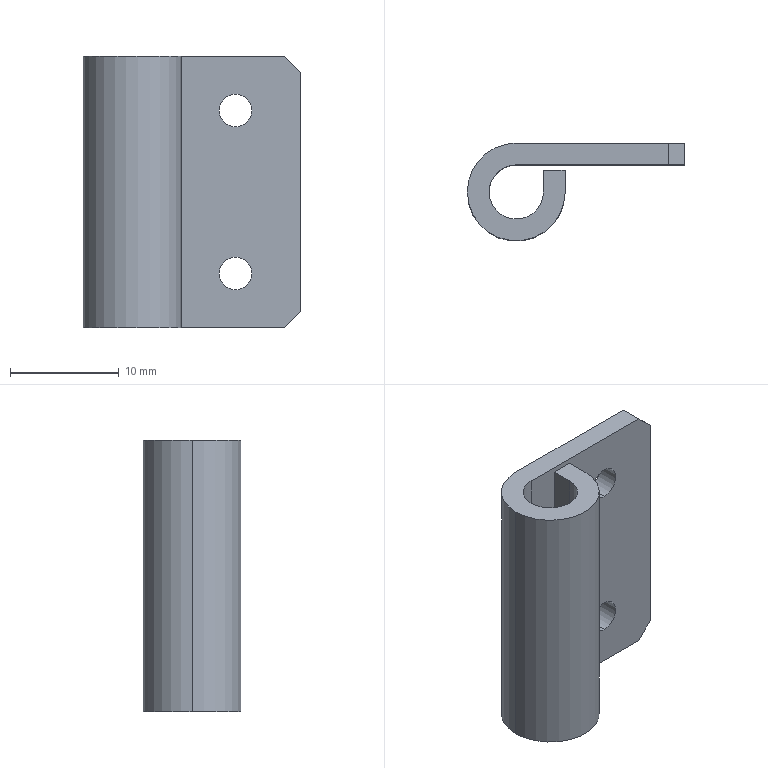Part | STEP file | 1 solid | 18 faces | box 20 x 9 x 25 mm | volume 1667 mm3 | plane 10 | cylinder 8 | commonest cylinder face diameters 3 x4 5 x2 9 x2
STEP:
#1=CARTESIAN_POINT('',(0.,0.,0.));
#2=DIRECTION('',(0.,0.,1.));
#3=DIRECTION('',(1.,0.,0.));
#4=AXIS2_PLACEMENT_3D('',#1,#2,#3);
#5=CARTESIAN_POINT('',(9.5,2.5,21.5));
#6=VERTEX_POINT('',#5);
#7=CARTESIAN_POINT('',(9.5,4.5,21.5));
#8=VERTEX_POINT('',#7);
#9=CARTESIAN_POINT('',(9.5,-4.5,21.5));
#10=DIRECTION('',(0.,1.,0.));
#11=VECTOR('',#10,1.);
#12=LINE('',#9,#11);
#13=CARTESIAN_POINT('',(9.5,-4.5,20.));
#14=DIRECTION('',(0.,1.,0.));
#15=DIRECTION('',(0.,0.,1.));
#16=AXIS2_PLACEMENT_3D('',#13,#14,#15);
#17=CYLINDRICAL_SURFACE('',#16,1.5);
#18=CARTESIAN_POINT('',(6.283,0.));
#19=DIRECTION('',(0.,1.));
#20=VECTOR('',#19,1.);
#21=LINE('',#18,#20);
#22=(GEOMETRIC_REPRESENTATION_CONTEXT(2)PARAMETRIC_REPRESENTATION_CONTEXT()REPRESENTATION_CONTEXT('',''));
#23=DEFINITIONAL_REPRESENTATION('',(#21),#22);
#24=PCURVE('',#17,#23);
#25=CARTESIAN_POINT('',(9.5,-4.5,20.));
#26=DIRECTION('',(0.,1.,0.));
#27=DIRECTION('',(0.,0.,1.));
#28=AXIS2_PLACEMENT_3D('',#25,#26,#27);
#29=CYLINDRICAL_SURFACE('',#28,1.5);
#30=CARTESIAN_POINT('',(0.,0.));
#31=DIRECTION('',(0.,1.));
#32=VECTOR('',#31,1.);
#33=LINE('',#30,#32);
#34=(GEOMETRIC_REPRESENTATION_CONTEXT(2)PARAMETRIC_REPRESENTATION_CONTEXT()REPRESENTATION_CONTEXT('',''));
#35=DEFINITIONAL_REPRESENTATION('',(#33),#34);
#36=PCURVE('',#29,#35);
#37=SURFACE_CURVE('',#12,(#24,#36),.PCURVE_S1.);
#38=EDGE_CURVE('',#6,#8,#37,.T.);
#39=ORIENTED_EDGE('',*,*,#38,.T.);
#40=CARTESIAN_POINT('',(9.5,4.5,18.5));
#41=VERTEX_POINT('',#40);
#42=CARTESIAN_POINT('',(9.5,4.5,20.));
#43=DIRECTION('',(0.,1.,0.));
#44=DIRECTION('',(0.,0.,-1.));
#45=AXIS2_PLACEMENT_3D('',#42,#43,#44);
#46=CIRCLE('',#45,1.5);
#47=CARTESIAN_POINT('',(3.142,9.));
#48=DIRECTION('',(1.,0.));
#49=VECTOR('',#48,1.);
#50=LINE('',#47,#49);
#51=(GEOMETRIC_REPRESENTATION_CONTEXT(2)PARAMETRIC_REPRESENTATION_CONTEXT()REPRESENTATION_CONTEXT('',''));
#52=DEFINITIONAL_REPRESENTATION('',(#50),#51);
#53=PCURVE('',#17,#52);
#54=CARTESIAN_POINT('',(0.,4.5,25.));
#55=DIRECTION('',(0.,-1.,0.));
#56=DIRECTION('',(0.,0.,-1.));
#57=AXIS2_PLACEMENT_3D('',#54,#55,#56);
#58=PLANE('',#57);
#59=CARTESIAN_POINT('',(6.5,9.5));
#60=CARTESIAN_POINT('',(6.5,6.902));
#61=CARTESIAN_POINT('',(4.25,8.201));
#62=CARTESIAN_POINT('',(2.,9.5));
#63=CARTESIAN_POINT('',(4.25,10.799));
#64=CARTESIAN_POINT('',(6.5,12.098));
#65=CARTESIAN_POINT('',(6.5,9.5));
#66=(BOUNDED_CURVE()B_SPLINE_CURVE(2,(#59,#60,#61,#62,#63,#64,#65),.UNSPECIFIED.,.T.,.F.)B_SPLINE_CURVE_WITH_KNOTS((1,2,2,2,2,1),(-2.094,0.,2.094,4.189,6.283,8.378),.UNSPECIFIED.)CURVE()GEOMETRIC_REPRESENTATION_ITEM()RATIONAL_B_SPLINE_CURVE((1.,0.5,1.,0.5,1.,0.5,1.))REPRESENTATION_ITEM(''));
#67=(GEOMETRIC_REPRESENTATION_CONTEXT(2)PARAMETRIC_REPRESENTATION_CONTEXT()REPRESENTATION_CONTEXT('',''));
#68=DEFINITIONAL_REPRESENTATION('',(#66),#67);
#69=PCURVE('',#58,#68);
#70=SURFACE_CURVE('',#46,(#53,#69),.PCURVE_S1.);
#71=EDGE_CURVE('',#41,#8,#70,.T.);
#72=ORIENTED_EDGE('',*,*,#71,.F.);
#73=CARTESIAN_POINT('',(9.5,2.5,18.5));
#74=VERTEX_POINT('',#73);
#75=CARTESIAN_POINT('',(9.5,-4.5,18.5));
#76=DIRECTION('',(0.,1.,0.));
#77=VECTOR('',#76,1.);
#78=LINE('',#75,#77);
#79=CARTESIAN_POINT('',(3.142,0.));
#80=DIRECTION('',(0.,1.));
#81=VECTOR('',#80,1.);
#82=LINE('',#79,#81);
#83=(GEOMETRIC_REPRESENTATION_CONTEXT(2)PARAMETRIC_REPRESENTATION_CONTEXT()REPRESENTATION_CONTEXT('',''));
#84=DEFINITIONAL_REPRESENTATION('',(#82),#83);
#85=PCURVE('',#17,#84);
#86=CARTESIAN_POINT('',(3.142,0.));
#87=DIRECTION('',(0.,1.));
#88=VECTOR('',#87,1.);
#89=LINE('',#86,#88);
#90=(GEOMETRIC_REPRESENTATION_CONTEXT(2)PARAMETRIC_REPRESENTATION_CONTEXT()REPRESENTATION_CONTEXT('',''));
#91=DEFINITIONAL_REPRESENTATION('',(#89),#90);
#92=PCURVE('',#29,#91);
#93=SURFACE_CURVE('',#78,(#85,#92),.PCURVE_S1.);
#94=EDGE_CURVE('',#74,#41,#93,.T.);
#95=ORIENTED_EDGE('',*,*,#94,.F.);
#96=CARTESIAN_POINT('',(9.5,2.5,20.));
#97=DIRECTION('',(0.,1.,0.));
#98=DIRECTION('',(-1.,0.,0.));
#99=AXIS2_PLACEMENT_3D('',#96,#97,#98);
#100=CIRCLE('',#99,1.5);
#101=CARTESIAN_POINT('',(-1.571,7.));
#102=DIRECTION('',(1.,0.));
#103=VECTOR('',#102,1.);
#104=LINE('',#101,#103);
#105=(GEOMETRIC_REPRESENTATION_CONTEXT(2)PARAMETRIC_REPRESENTATION_CONTEXT()REPRESENTATION_CONTEXT('',''));
#106=DEFINITIONAL_REPRESENTATION('',(#104),#105);
#107=PCURVE('',#17,#106);
#108=CARTESIAN_POINT('',(15.5,2.5,25.));
#109=DIRECTION('',(0.,1.,0.));
#110=DIRECTION('',(1.,0.,0.));
#111=AXIS2_PLACEMENT_3D('',#108,#109,#110);
#112=PLANE('',#111);
#113=CARTESIAN_POINT('',(-6.,5.));
#114=DIRECTION('',(-1.,0.));
#115=AXIS2_PLACEMENT_2D('',#113,#114);
#116=CIRCLE('',#115,1.5);
#117=(GEOMETRIC_REPRESENTATION_CONTEXT(2)PARAMETRIC_REPRESENTATION_CONTEXT()REPRESENTATION_CONTEXT('',''));
#118=DEFINITIONAL_REPRESENTATION('',(#116),#117);
#119=PCURVE('',#112,#118);
#120=SURFACE_CURVE('',#100,(#107,#119),.PCURVE_S1.);
#121=EDGE_CURVE('',#74,#6,#120,.T.);
#122=ORIENTED_EDGE('',*,*,#121,.T.);
#123=EDGE_LOOP('',(#39,#72,#95,#122));
#124=FACE_BOUND('',#123,.F.);
#125=ADVANCED_FACE('',(#124),#17,.F.);
#126=CARTESIAN_POINT('',(9.5,2.5,6.5));
#127=VERTEX_POINT('',#126);
#128=CARTESIAN_POINT('',(9.5,4.5,6.5));
#129=VERTEX_POINT('',#128);
#130=CARTESIAN_POINT('',(9.5,-4.5,6.5));
#131=DIRECTION('',(0.,1.,0.));
#132=VECTOR('',#131,1.);
#133=LINE('',#130,#132);
#134=CARTESIAN_POINT('',(9.5,-4.5,5.));
#135=DIRECTION('',(0.,1.,0.));
#136=DIRECTION('',(0.,0.,1.));
#137=AXIS2_PLACEMENT_3D('',#134,#135,#136);
#138=CYLINDRICAL_SURFACE('',#137,1.5);
#139=CARTESIAN_POINT('',(6.283,0.));
#140=DIRECTION('',(0.,1.));
#141=VECTOR('',#140,1.);
#142=LINE('',#139,#141);
#143=(GEOMETRIC_REPRESENTATION_CONTEXT(2)PARAMETRIC_REPRESENTATION_CONTEXT()REPRESENTATION_CONTEXT('',''));
#144=DEFINITIONAL_REPRESENTATION('',(#142),#143);
#145=PCURVE('',#138,#144);
#146=CARTESIAN_POINT('',(9.5,-4.5,5.));
#147=DIRECTION('',(0.,1.,0.));
#148=DIRECTION('',(0.,0.,1.));
#149=AXIS2_PLACEMENT_3D('',#146,#147,#148);
#150=CYLINDRICAL_SURFACE('',#149,1.5);
#151=CARTESIAN_POINT('',(0.,0.));
#152=DIRECTION('',(0.,1.));
#153=VECTOR('',#152,1.);
#154=LINE('',#151,#153);
#155=(GEOMETRIC_REPRESENTATION_CONTEXT(2)PARAMETRIC_REPRESENTATION_CONTEXT()REPRESENTATION_CONTEXT('',''));
#156=DEFINITIONAL_REPRESENTATION('',(#154),#155);
#157=PCURVE('',#150,#156);
#158=SURFACE_CURVE('',#133,(#145,#157),.PCURVE_S1.);
#159=EDGE_CURVE('',#127,#129,#158,.T.);
#160=ORIENTED_EDGE('',*,*,#159,.T.);
#161=CARTESIAN_POINT('',(9.5,4.5,3.5));
#162=VERTEX_POINT('',#161);
#163=CARTESIAN_POINT('',(9.5,4.5,5.));
#164=DIRECTION('',(0.,1.,0.));
#165=DIRECTION('',(0.,0.,1.));
#166=AXIS2_PLACEMENT_3D('',#163,#164,#165);
#167=CIRCLE('',#166,1.5);
#168=CARTESIAN_POINT('',(0.,9.));
#169=DIRECTION('',(1.,0.));
#170=VECTOR('',#169,1.);
#171=LINE('',#168,#170);
#172=(GEOMETRIC_REPRESENTATION_CONTEXT(2)PARAMETRIC_REPRESENTATION_CONTEXT()REPRESENTATION_CONTEXT('',''));
#173=DEFINITIONAL_REPRESENTATION('',(#171),#172);
#174=PCURVE('',#138,#173);
#175=CARTESIAN_POINT('',(18.5,9.5));
#176=CARTESIAN_POINT('',(18.5,12.098));
#177=CARTESIAN_POINT('',(20.75,10.799));
#178=CARTESIAN_POINT('',(23.,9.5));
#179=CARTESIAN_POINT('',(20.75,8.201));
#180=CARTESIAN_POINT('',(18.5,6.902));
#181=CARTESIAN_POINT('',(18.5,9.5));
#182=(BOUNDED_CURVE()B_SPLINE_CURVE(2,(#175,#176,#177,#178,#179,#180,#181),.UNSPECIFIED.,.T.,.F.)B_SPLINE_CURVE_WITH_KNOTS((1,2,2,2,2,1),(-2.094,0.,2.094,4.189,6.283,8.378),.UNSPECIFIED.)CURVE()GEOMETRIC_REPRESENTATION_ITEM()RATIONAL_B_SPLINE_CURVE((1.,0.5,1.,0.5,1.,0.5,1.))REPRESENTATION_ITEM(''));
#183=(GEOMETRIC_REPRESENTATION_CONTEXT(2)PARAMETRIC_REPRESENTATION_CONTEXT()REPRESENTATION_CONTEXT('',''));
#184=DEFINITIONAL_REPRESENTATION('',(#182),#183);
#185=PCURVE('',#58,#184);
#186=SURFACE_CURVE('',#167,(#174,#185),.PCURVE_S1.);
#187=EDGE_CURVE('',#162,#129,#186,.T.);
#188=ORIENTED_EDGE('',*,*,#187,.F.);
#189=CARTESIAN_POINT('',(9.5,2.5,3.5));
#190=VERTEX_POINT('',#189);
#191=CARTESIAN_POINT('',(9.5,-4.5,3.5));
#192=DIRECTION('',(0.,1.,0.));
#193=VECTOR('',#192,1.);
#194=LINE('',#191,#193);
#195=CARTESIAN_POINT('',(3.142,0.));
#196=DIRECTION('',(0.,1.));
#197=VECTOR('',#196,1.);
#198=LINE('',#195,#197);
#199=(GEOMETRIC_REPRESENTATION_CONTEXT(2)PARAMETRIC_REPRESENTATION_CONTEXT()REPRESENTATION_CONTEXT('',''));
#200=DEFINITIONAL_REPRESENTATION('',(#198),#199);
#201=PCURVE('',#138,#200);
#202=CARTESIAN_POINT('',(3.142,0.));
#203=DIRECTION('',(0.,1.));
#204=VECTOR('',#203,1.);
#205=LINE('',#202,#204);
#206=(GEOMETRIC_REPRESENTATION_CONTEXT(2)PARAMETRIC_REPRESENTATION_CONTEXT()REPRESENTATION_CONTEXT('',''));
#207=DEFINITIONAL_REPRESENTATION('',(#205),#206);
#208=PCURVE('',#150,#207);
#209=SURFACE_CURVE('',#194,(#201,#208),.PCURVE_S1.);
#210=EDGE_CURVE('',#190,#162,#209,.T.);
#211=ORIENTED_EDGE('',*,*,#210,.F.);
#212=CARTESIAN_POINT('',(9.5,2.5,5.));
#213=DIRECTION('',(0.,1.,0.));
#214=DIRECTION('',(-1.,0.,0.));
#215=AXIS2_PLACEMENT_3D('',#212,#213,#214);
#216=CIRCLE('',#215,1.5);
#217=CARTESIAN_POINT('',(-1.571,7.));
#218=DIRECTION('',(1.,0.));
#219=VECTOR('',#218,1.);
#220=LINE('',#217,#219);
#221=(GEOMETRIC_REPRESENTATION_CONTEXT(2)PARAMETRIC_REPRESENTATION_CONTEXT()REPRESENTATION_CONTEXT('',''));
#222=DEFINITIONAL_REPRESENTATION('',(#220),#221);
#223=PCURVE('',#138,#222);
#224=CARTESIAN_POINT('',(-6.,20.));
#225=DIRECTION('',(-1.,0.));
#226=AXIS2_PLACEMENT_2D('',#224,#225);
#227=CIRCLE('',#226,1.5);
#228=(GEOMETRIC_REPRESENTATION_CONTEXT(2)PARAMETRIC_REPRESENTATION_CONTEXT()REPRESENTATION_CONTEXT('',''));
#229=DEFINITIONAL_REPRESENTATION('',(#227),#228);
#230=PCURVE('',#112,#229);
#231=SURFACE_CURVE('',#216,(#223,#230),.PCURVE_S1.);
#232=EDGE_CURVE('',#190,#127,#231,.T.);
#233=ORIENTED_EDGE('',*,*,#232,.T.);
#234=EDGE_LOOP('',(#160,#188,#211,#233));
#235=FACE_BOUND('',#234,.F.);
#236=ADVANCED_FACE('',(#235),#138,.F.);
#237=CARTESIAN_POINT('',(0.,2.5,25.));
#238=VERTEX_POINT('',#237);
#239=CARTESIAN_POINT('',(0.,2.5,0.));
#240=VERTEX_POINT('',#239);
#241=CARTESIAN_POINT('',(0.,2.5,25.));
#242=DIRECTION('',(0.,0.,-1.));
#243=VECTOR('',#242,1.);
#244=LINE('',#241,#243);
#245=CARTESIAN_POINT('',(0.,0.,25.));
#246=DIRECTION('',(0.,0.,-1.));
#247=DIRECTION('',(-1.,0.,0.));
#248=AXIS2_PLACEMENT_3D('',#245,#246,#247);
#249=CYLINDRICAL_SURFACE('',#248,2.5);
#250=CARTESIAN_POINT('',(1.571,0.));
#251=DIRECTION('',(0.,1.));
#252=VECTOR('',#251,1.);
#253=LINE('',#250,#252);
#254=(GEOMETRIC_REPRESENTATION_CONTEXT(2)PARAMETRIC_REPRESENTATION_CONTEXT()REPRESENTATION_CONTEXT('',''));
#255=DEFINITIONAL_REPRESENTATION('',(#253),#254);
#256=PCURVE('',#249,#255);
#257=CARTESIAN_POINT('',(-15.5,0.));
#258=DIRECTION('',(0.,1.));
#259=VECTOR('',#258,1.);
#260=LINE('',#257,#259);
#261=(GEOMETRIC_REPRESENTATION_CONTEXT(2)PARAMETRIC_REPRESENTATION_CONTEXT()REPRESENTATION_CONTEXT('',''));
#262=DEFINITIONAL_REPRESENTATION('',(#260),#261);
#263=PCURVE('',#112,#262);
#264=SURFACE_CURVE('',#244,(#256,#263),.PCURVE_S1.);
#265=EDGE_CURVE('',#238,#240,#264,.T.);
#266=ORIENTED_EDGE('',*,*,#265,.T.);
#267=CARTESIAN_POINT('',(-2.5,0.,0.));
#268=VERTEX_POINT('',#267);
#269=CARTESIAN_POINT('',(0.,0.,0.));
#270=DIRECTION('',(0.,0.,-1.));
#271=DIRECTION('',(1.,0.,0.));
#272=AXIS2_PLACEMENT_3D('',#269,#270,#271);
#273=CIRCLE('',#272,2.5);
#274=CARTESIAN_POINT('',(-3.142,25.));
#275=DIRECTION('',(1.,0.));
#276=VECTOR('',#275,1.);
#277=LINE('',#274,#276);
#278=(GEOMETRIC_REPRESENTATION_CONTEXT(2)PARAMETRIC_REPRESENTATION_CONTEXT()REPRESENTATION_CONTEXT('',''));
#279=DEFINITIONAL_REPRESENTATION('',(#277),#278);
#280=PCURVE('',#249,#279);
#281=CARTESIAN_POINT('',(0.,0.,0.));
#282=DIRECTION('',(0.,0.,1.));
#283=DIRECTION('',(1.,0.,0.));
#284=AXIS2_PLACEMENT_3D('',#281,#282,#283);
#285=PLANE('',#284);
#286=CARTESIAN_POINT('',(2.5,0.));
#287=CARTESIAN_POINT('',(2.5,-4.33));
#288=CARTESIAN_POINT('',(-1.25,-2.165));
#289=CARTESIAN_POINT('',(-5.,0.));
#290=CARTESIAN_POINT('',(-1.25,2.165));
#291=CARTESIAN_POINT('',(2.5,4.33));
#292=CARTESIAN_POINT('',(2.5,0.));
#293=(BOUNDED_CURVE()B_SPLINE_CURVE(2,(#286,#287,#288,#289,#290,#291,#292),.UNSPECIFIED.,.T.,.F.)B_SPLINE_CURVE_WITH_KNOTS((1,2,2,2,2,1),(-2.094,0.,2.094,4.189,6.283,8.378),.UNSPECIFIED.)CURVE()GEOMETRIC_REPRESENTATION_ITEM()RATIONAL_B_SPLINE_CURVE((1.,0.5,1.,0.5,1.,0.5,1.))REPRESENTATION_ITEM(''));
#294=(GEOMETRIC_REPRESENTATION_CONTEXT(2)PARAMETRIC_REPRESENTATION_CONTEXT()REPRESENTATION_CONTEXT('',''));
#295=DEFINITIONAL_REPRESENTATION('',(#293),#294);
#296=PCURVE('',#285,#295);
#297=SURFACE_CURVE('',#273,(#280,#296),.PCURVE_S1.);
#298=EDGE_CURVE('',#268,#240,#297,.T.);
#299=ORIENTED_EDGE('',*,*,#298,.F.);
#300=CARTESIAN_POINT('',(-2.5,0.,25.));
#301=VERTEX_POINT('',#300);
#302=CARTESIAN_POINT('',(-2.5,0.,25.));
#303=DIRECTION('',(0.,0.,-1.));
#304=VECTOR('',#303,1.);
#305=LINE('',#302,#304);
#306=CARTESIAN_POINT('',(0.,0.));
#307=DIRECTION('',(0.,1.));
#308=VECTOR('',#307,1.);
#309=LINE('',#306,#308);
#310=(GEOMETRIC_REPRESENTATION_CONTEXT(2)PARAMETRIC_REPRESENTATION_CONTEXT()REPRESENTATION_CONTEXT('',''));
#311=DEFINITIONAL_REPRESENTATION('',(#309),#310);
#312=PCURVE('',#249,#311);
#313=CARTESIAN_POINT('',(0.,0.,25.));
#314=DIRECTION('',(0.,0.,-1.));
#315=DIRECTION('',(-1.,0.,0.));
#316=AXIS2_PLACEMENT_3D('',#313,#314,#315);
#317=CYLINDRICAL_SURFACE('',#316,2.5);
#318=CARTESIAN_POINT('',(6.283,0.));
#319=DIRECTION('',(0.,1.));
#320=VECTOR('',#319,1.);
#321=LINE('',#318,#320);
#322=(GEOMETRIC_REPRESENTATION_CONTEXT(2)PARAMETRIC_REPRESENTATION_CONTEXT()REPRESENTATION_CONTEXT('',''));
#323=DEFINITIONAL_REPRESENTATION('',(#321),#322);
#324=PCURVE('',#317,#323);
#325=SURFACE_CURVE('',#305,(#312,#324),.PCURVE_S1.);
#326=EDGE_CURVE('',#301,#268,#325,.T.);
#327=ORIENTED_EDGE('',*,*,#326,.F.);
#328=CARTESIAN_POINT('',(0.,0.,25.));
#329=DIRECTION('',(0.,0.,-1.));
#330=DIRECTION('',(1.,0.,0.));
#331=AXIS2_PLACEMENT_3D('',#328,#329,#330);
#332=CIRCLE('',#331,2.5);
#333=CARTESIAN_POINT('',(-3.142,0.));
#334=DIRECTION('',(1.,0.));
#335=VECTOR('',#334,1.);
#336=LINE('',#333,#335);
#337=(GEOMETRIC_REPRESENTATION_CONTEXT(2)PARAMETRIC_REPRESENTATION_CONTEXT()REPRESENTATION_CONTEXT('',''));
#338=DEFINITIONAL_REPRESENTATION('',(#336),#337);
#339=PCURVE('',#249,#338);
#340=CARTESIAN_POINT('',(0.,0.,25.));
#341=DIRECTION('',(0.,0.,1.));
#342=DIRECTION('',(1.,0.,0.));
#343=AXIS2_PLACEMENT_3D('',#340,#341,#342);
#344=PLANE('',#343);
#345=CARTESIAN_POINT('',(2.5,0.));
#346=CARTESIAN_POINT('',(2.5,-4.33));
#347=CARTESIAN_POINT('',(-1.25,-2.165));
#348=CARTESIAN_POINT('',(-5.,0.));
#349=CARTESIAN_POINT('',(-1.25,2.165));
#350=CARTESIAN_POINT('',(2.5,4.33));
#351=CARTESIAN_POINT('',(2.5,0.));
#352=(BOUNDED_CURVE()B_SPLINE_CURVE(2,(#345,#346,#347,#348,#349,#350,#351),.UNSPECIFIED.,.T.,.F.)B_SPLINE_CURVE_WITH_KNOTS((1,2,2,2,2,1),(-2.094,0.,2.094,4.189,6.283,8.378),.UNSPECIFIED.)CURVE()GEOMETRIC_REPRESENTATION_ITEM()RATIONAL_B_SPLINE_CURVE((1.,0.5,1.,0.5,1.,0.5,1.))REPRESENTATION_ITEM(''));
#353=(GEOMETRIC_REPRESENTATION_CONTEXT(2)PARAMETRIC_REPRESENTATION_CONTEXT()REPRESENTATION_CONTEXT('',''));
#354=DEFINITIONAL_REPRESENTATION('',(#352),#353);
#355=PCURVE('',#344,#354);
#356=SURFACE_CURVE('',#332,(#339,#355),.PCURVE_S1.);
#357=EDGE_CURVE('',#301,#238,#356,.T.);
#358=ORIENTED_EDGE('',*,*,#357,.T.);
#359=EDGE_LOOP('',(#266,#299,#327,#358));
#360=FACE_BOUND('',#359,.F.);
#361=ADVANCED_FACE('',(#360),#249,.F.);
#362=CARTESIAN_POINT('',(-4.5,0.,25.));
#363=VERTEX_POINT('',#362);
#364=CARTESIAN_POINT('',(4.5,0.,25.));
#365=VERTEX_POINT('',#364);
#366=CARTESIAN_POINT('',(0.,0.,25.));
#367=DIRECTION('',(0.,0.,1.));
#368=DIRECTION('',(1.,0.,0.));
#369=AXIS2_PLACEMENT_3D('',#366,#367,#368);
#370=CIRCLE('',#369,4.5);
#371=CARTESIAN_POINT('',(0.,0.,25.));
#372=DIRECTION('',(0.,0.,-1.));
#373=DIRECTION('',(-1.,0.,0.));
#374=AXIS2_PLACEMENT_3D('',#371,#372,#373);
#375=CYLINDRICAL_SURFACE('',#374,4.5);
#376=CARTESIAN_POINT('',(9.425,0.));
#377=DIRECTION('',(-1.,0.));
#378=VECTOR('',#377,1.);
#379=LINE('',#376,#378);
#380=(GEOMETRIC_REPRESENTATION_CONTEXT(2)PARAMETRIC_REPRESENTATION_CONTEXT()REPRESENTATION_CONTEXT('',''));
#381=DEFINITIONAL_REPRESENTATION('',(#379),#380);
#382=PCURVE('',#375,#381);
#383=CARTESIAN_POINT('',(0.,0.));
#384=DIRECTION('',(1.,0.));
#385=AXIS2_PLACEMENT_2D('',#383,#384);
#386=CIRCLE('',#385,4.5);
#387=(GEOMETRIC_REPRESENTATION_CONTEXT(2)PARAMETRIC_REPRESENTATION_CONTEXT()REPRESENTATION_CONTEXT('',''));
#388=DEFINITIONAL_REPRESENTATION('',(#386),#387);
#389=PCURVE('',#344,#388);
#390=SURFACE_CURVE('',#370,(#382,#389),.PCURVE_S1.);
#391=EDGE_CURVE('',#363,#365,#390,.T.);
#392=ORIENTED_EDGE('',*,*,#391,.F.);
#393=CARTESIAN_POINT('',(-4.5,0.,0.));
#394=VERTEX_POINT('',#393);
#395=CARTESIAN_POINT('',(-4.5,0.,25.));
#396=DIRECTION('',(0.,0.,-1.));
#397=VECTOR('',#396,1.);
#398=LINE('',#395,#397);
#399=CARTESIAN_POINT('',(6.283,0.));
#400=DIRECTION('',(0.,1.));
#401=VECTOR('',#400,1.);
#402=LINE('',#399,#401);
#403=(GEOMETRIC_REPRESENTATION_CONTEXT(2)PARAMETRIC_REPRESENTATION_CONTEXT()REPRESENTATION_CONTEXT('',''));
#404=DEFINITIONAL_REPRESENTATION('',(#402),#403);
#405=PCURVE('',#375,#404);
#406=CARTESIAN_POINT('',(0.,0.,25.));
#407=DIRECTION('',(0.,0.,-1.));
#408=DIRECTION('',(-1.,0.,0.));
#409=AXIS2_PLACEMENT_3D('',#406,#407,#408);
#410=CYLINDRICAL_SURFACE('',#409,4.5);
#411=CARTESIAN_POINT('',(0.,0.));
#412=DIRECTION('',(0.,1.));
#413=VECTOR('',#412,1.);
#414=LINE('',#411,#413);
#415=(GEOMETRIC_REPRESENTATION_CONTEXT(2)PARAMETRIC_REPRESENTATION_CONTEXT()REPRESENTATION_CONTEXT('',''));
#416=DEFINITIONAL_REPRESENTATION('',(#414),#415);
#417=PCURVE('',#410,#416);
#418=SURFACE_CURVE('',#398,(#405,#417),.PCURVE_S1.);
#419=EDGE_CURVE('',#363,#394,#418,.T.);
#420=ORIENTED_EDGE('',*,*,#419,.T.);
#421=CARTESIAN_POINT('',(4.5,0.,0.));
#422=VERTEX_POINT('',#421);
#423=CARTESIAN_POINT('',(0.,0.,0.));
#424=DIRECTION('',(0.,0.,1.));
#425=DIRECTION('',(1.,0.,0.));
#426=AXIS2_PLACEMENT_3D('',#423,#424,#425);
#427=CIRCLE('',#426,4.5);
#428=CARTESIAN_POINT('',(9.425,25.));
#429=DIRECTION('',(-1.,0.));
#430=VECTOR('',#429,1.);
#431=LINE('',#428,#430);
#432=(GEOMETRIC_REPRESENTATION_CONTEXT(2)PARAMETRIC_REPRESENTATION_CONTEXT()REPRESENTATION_CONTEXT('',''));
#433=DEFINITIONAL_REPRESENTATION('',(#431),#432);
#434=PCURVE('',#375,#433);
#435=CARTESIAN_POINT('',(0.,0.));
#436=DIRECTION('',(1.,0.));
#437=AXIS2_PLACEMENT_2D('',#435,#436);
#438=CIRCLE('',#437,4.5);
#439=(GEOMETRIC_REPRESENTATION_CONTEXT(2)PARAMETRIC_REPRESENTATION_CONTEXT()REPRESENTATION_CONTEXT('',''));
#440=DEFINITIONAL_REPRESENTATION('',(#438),#439);
#441=PCURVE('',#285,#440);
#442=SURFACE_CURVE('',#427,(#434,#441),.PCURVE_S1.);
#443=EDGE_CURVE('',#394,#422,#442,.T.);
#444=ORIENTED_EDGE('',*,*,#443,.T.);
#445=CARTESIAN_POINT('',(4.5,0.,25.));
#446=DIRECTION('',(0.,0.,-1.));
#447=VECTOR('',#446,1.);
#448=LINE('',#445,#447);
#449=CARTESIAN_POINT('',(3.142,0.));
#450=DIRECTION('',(0.,1.));
#451=VECTOR('',#450,1.);
#452=LINE('',#449,#451);
#453=(GEOMETRIC_REPRESENTATION_CONTEXT(2)PARAMETRIC_REPRESENTATION_CONTEXT()REPRESENTATION_CONTEXT('',''));
#454=DEFINITIONAL_REPRESENTATION('',(#452),#453);
#455=PCURVE('',#375,#454);
#456=CARTESIAN_POINT('',(4.5,0.,25.));
#457=DIRECTION('',(-1.,0.,0.));
#458=DIRECTION('',(0.,0.,1.));
#459=AXIS2_PLACEMENT_3D('',#456,#457,#458);
#460=PLANE('',#459);
#461=CARTESIAN_POINT('',(0.,0.));
#462=DIRECTION('',(-1.,0.));
#463=VECTOR('',#462,1.);
#464=LINE('',#461,#463);
#465=(GEOMETRIC_REPRESENTATION_CONTEXT(2)PARAMETRIC_REPRESENTATION_CONTEXT()REPRESENTATION_CONTEXT('',''));
#466=DEFINITIONAL_REPRESENTATION('',(#464),#465);
#467=PCURVE('',#460,#466);
#468=SURFACE_CURVE('',#448,(#455,#467),.PCURVE_S1.);
#469=EDGE_CURVE('',#365,#422,#468,.T.);
#470=ORIENTED_EDGE('',*,*,#469,.F.);
#471=EDGE_LOOP('',(#392,#420,#444,#470));
#472=FACE_BOUND('',#471,.T.);
#473=ADVANCED_FACE('',(#472),#375,.T.);
#474=CARTESIAN_POINT('',(15.5,2.5,23.5));
#475=VERTEX_POINT('',#474);
#476=CARTESIAN_POINT('',(15.5,4.5,23.5));
#477=VERTEX_POINT('',#476);
#478=CARTESIAN_POINT('',(15.5,-4.5,23.5));
#479=DIRECTION('',(0.,1.,0.));
#480=VECTOR('',#479,1.);
#481=LINE('',#478,#480);
#482=CARTESIAN_POINT('',(14.,-4.5,25.));
#483=DIRECTION('',(-0.7071,0.,-0.7071));
#484=DIRECTION('',(-0.7071,0.,0.7071));
#485=AXIS2_PLACEMENT_3D('',#482,#483,#484);
#486=PLANE('',#485);
#487=CARTESIAN_POINT('',(-2.121,0.));
#488=DIRECTION('',(0.,1.));
#489=VECTOR('',#488,1.);
#490=LINE('',#487,#489);
#491=(GEOMETRIC_REPRESENTATION_CONTEXT(2)PARAMETRIC_REPRESENTATION_CONTEXT()REPRESENTATION_CONTEXT('',''));
#492=DEFINITIONAL_REPRESENTATION('',(#490),#491);
#493=PCURVE('',#486,#492);
#494=CARTESIAN_POINT('',(15.5,4.5,25.));
#495=DIRECTION('',(-1.,0.,0.));
#496=DIRECTION('',(0.,1.,0.));
#497=AXIS2_PLACEMENT_3D('',#494,#495,#496);
#498=PLANE('',#497);
#499=CARTESIAN_POINT('',(-9.,1.5));
#500=DIRECTION('',(1.,0.));
#501=VECTOR('',#500,1.);
#502=LINE('',#499,#501);
#503=(GEOMETRIC_REPRESENTATION_CONTEXT(2)PARAMETRIC_REPRESENTATION_CONTEXT()REPRESENTATION_CONTEXT('',''));
#504=DEFINITIONAL_REPRESENTATION('',(#502),#503);
#505=PCURVE('',#498,#504);
#506=SURFACE_CURVE('',#481,(#493,#505),.PCURVE_S1.);
#507=EDGE_CURVE('',#475,#477,#506,.T.);
#508=ORIENTED_EDGE('',*,*,#507,.T.);
#509=CARTESIAN_POINT('',(14.,4.5,25.));
#510=VERTEX_POINT('',#509);
#511=CARTESIAN_POINT('',(14.,4.5,25.));
#512=DIRECTION('',(-0.7071,0.,0.7071));
#513=VECTOR('',#512,1.);
#514=LINE('',#511,#513);
#515=CARTESIAN_POINT('',(0.,9.));
#516=DIRECTION('',(1.,0.));
#517=VECTOR('',#516,1.);
#518=LINE('',#515,#517);
#519=(GEOMETRIC_REPRESENTATION_CONTEXT(2)PARAMETRIC_REPRESENTATION_CONTEXT()REPRESENTATION_CONTEXT('',''));
#520=DEFINITIONAL_REPRESENTATION('',(#518),#519);
#521=PCURVE('',#486,#520);
#522=CARTESIAN_POINT('',(0.,14.));
#523=DIRECTION('',(-0.7071,-0.7071));
#524=VECTOR('',#523,1.);
#525=LINE('',#522,#524);
#526=(GEOMETRIC_REPRESENTATION_CONTEXT(2)PARAMETRIC_REPRESENTATION_CONTEXT()REPRESENTATION_CONTEXT('',''));
#527=DEFINITIONAL_REPRESENTATION('',(#525),#526);
#528=PCURVE('',#58,#527);
#529=SURFACE_CURVE('',#514,(#521,#528),.PCURVE_S1.);
#530=EDGE_CURVE('',#477,#510,#529,.T.);
#531=ORIENTED_EDGE('',*,*,#530,.T.);
#532=CARTESIAN_POINT('',(14.,2.5,25.));
#533=VERTEX_POINT('',#532);
#534=CARTESIAN_POINT('',(14.,0.,25.));
#535=DIRECTION('',(0.,-1.,0.));
#536=VECTOR('',#535,1.);
#537=LINE('',#534,#536);
#538=CARTESIAN_POINT('',(0.,4.5));
#539=DIRECTION('',(0.,-1.));
#540=VECTOR('',#539,1.);
#541=LINE('',#538,#540);
#542=(GEOMETRIC_REPRESENTATION_CONTEXT(2)PARAMETRIC_REPRESENTATION_CONTEXT()REPRESENTATION_CONTEXT('',''));
#543=DEFINITIONAL_REPRESENTATION('',(#541),#542);
#544=PCURVE('',#486,#543);
#545=CARTESIAN_POINT('',(14.,0.));
#546=DIRECTION('',(0.,-1.));
#547=VECTOR('',#546,1.);
#548=LINE('',#545,#547);
#549=(GEOMETRIC_REPRESENTATION_CONTEXT(2)PARAMETRIC_REPRESENTATION_CONTEXT()REPRESENTATION_CONTEXT('',''));
#550=DEFINITIONAL_REPRESENTATION('',(#548),#549);
#551=PCURVE('',#344,#550);
#552=SURFACE_CURVE('',#537,(#544,#551),.PCURVE_S1.);
#553=EDGE_CURVE('',#510,#533,#552,.T.);
#554=ORIENTED_EDGE('',*,*,#553,.T.);
#555=CARTESIAN_POINT('',(14.75,2.5,24.25));
#556=DIRECTION('',(-0.7071,0.,0.7071));
#557=VECTOR('',#556,1.);
#558=LINE('',#555,#557);
#559=CARTESIAN_POINT('',(-1.061,7.));
#560=DIRECTION('',(1.,0.));
#561=VECTOR('',#560,1.);
#562=LINE('',#559,#561);
#563=(GEOMETRIC_REPRESENTATION_CONTEXT(2)PARAMETRIC_REPRESENTATION_CONTEXT()REPRESENTATION_CONTEXT('',''));
#564=DEFINITIONAL_REPRESENTATION('',(#562),#563);
#565=PCURVE('',#486,#564);
#566=CARTESIAN_POINT('',(-0.75,0.75));
#567=DIRECTION('',(-0.7071,-0.7071));
#568=VECTOR('',#567,1.);
#569=LINE('',#566,#568);
#570=(GEOMETRIC_REPRESENTATION_CONTEXT(2)PARAMETRIC_REPRESENTATION_CONTEXT()REPRESENTATION_CONTEXT('',''));
#571=DEFINITIONAL_REPRESENTATION('',(#569),#570);
#572=PCURVE('',#112,#571);
#573=SURFACE_CURVE('',#558,(#565,#572),.PCURVE_S1.);
#574=EDGE_CURVE('',#475,#533,#573,.T.);
#575=ORIENTED_EDGE('',*,*,#574,.F.);
#576=EDGE_LOOP('',(#508,#531,#554,#575));
#577=FACE_BOUND('',#576,.T.);
#578=ADVANCED_FACE('',(#577),#486,.F.);
#579=CARTESIAN_POINT('',(14.,4.5,0.));
#580=VERTEX_POINT('',#579);
#581=CARTESIAN_POINT('',(14.,2.5,0.));
#582=VERTEX_POINT('',#581);
#583=CARTESIAN_POINT('',(14.,0.,0.));
#584=DIRECTION('',(0.,-1.,0.));
#585=VECTOR('',#584,1.);
#586=LINE('',#583,#585);
#587=CARTESIAN_POINT('',(14.,-4.5,0.));
#588=DIRECTION('',(-0.7071,0.,0.7071));
#589=DIRECTION('',(0.,1.,0.));
#590=AXIS2_PLACEMENT_3D('',#587,#588,#589);
#591=PLANE('',#590);
#592=CARTESIAN_POINT('',(4.5,0.));
#593=DIRECTION('',(-1.,0.));
#594=VECTOR('',#593,1.);
#595=LINE('',#592,#594);
#596=(GEOMETRIC_REPRESENTATION_CONTEXT(2)PARAMETRIC_REPRESENTATION_CONTEXT()REPRESENTATION_CONTEXT('',''));
#597=DEFINITIONAL_REPRESENTATION('',(#595),#596);
#598=PCURVE('',#591,#597);
#599=CARTESIAN_POINT('',(14.,0.));
#600=DIRECTION('',(0.,-1.));
#601=VECTOR('',#600,1.);
#602=LINE('',#599,#601);
#603=(GEOMETRIC_REPRESENTATION_CONTEXT(2)PARAMETRIC_REPRESENTATION_CONTEXT()REPRESENTATION_CONTEXT('',''));
#604=DEFINITIONAL_REPRESENTATION('',(#602),#603);
#605=PCURVE('',#285,#604);
#606=SURFACE_CURVE('',#586,(#598,#605),.PCURVE_S1.);
#607=EDGE_CURVE('',#580,#582,#606,.T.);
#608=ORIENTED_EDGE('',*,*,#607,.F.);
#609=CARTESIAN_POINT('',(15.5,4.5,1.5));
#610=VERTEX_POINT('',#609);
#611=CARTESIAN_POINT('',(14.,4.5,0.));
#612=DIRECTION('',(0.7071,0.,0.7071));
#613=VECTOR('',#612,1.);
#614=LINE('',#611,#613);
#615=CARTESIAN_POINT('',(9.,0.));
#616=DIRECTION('',(0.,-1.));
#617=VECTOR('',#616,1.);
#618=LINE('',#615,#617);
#619=(GEOMETRIC_REPRESENTATION_CONTEXT(2)PARAMETRIC_REPRESENTATION_CONTEXT()REPRESENTATION_CONTEXT('',''));
#620=DEFINITIONAL_REPRESENTATION('',(#618),#619);
#621=PCURVE('',#591,#620);
#622=CARTESIAN_POINT('',(25.,14.));
#623=DIRECTION('',(-0.7071,0.7071));
#624=VECTOR('',#623,1.);
#625=LINE('',#622,#624);
#626=(GEOMETRIC_REPRESENTATION_CONTEXT(2)PARAMETRIC_REPRESENTATION_CONTEXT()REPRESENTATION_CONTEXT('',''));
#627=DEFINITIONAL_REPRESENTATION('',(#625),#626);
#628=PCURVE('',#58,#627);
#629=SURFACE_CURVE('',#614,(#621,#628),.PCURVE_S1.);
#630=EDGE_CURVE('',#580,#610,#629,.T.);
#631=ORIENTED_EDGE('',*,*,#630,.T.);
#632=CARTESIAN_POINT('',(15.5,2.5,1.5));
#633=VERTEX_POINT('',#632);
#634=CARTESIAN_POINT('',(15.5,-4.5,1.5));
#635=DIRECTION('',(0.,1.,0.));
#636=VECTOR('',#635,1.);
#637=LINE('',#634,#636);
#638=CARTESIAN_POINT('',(0.,-2.121));
#639=DIRECTION('',(1.,0.));
#640=VECTOR('',#639,1.);
#641=LINE('',#638,#640);
#642=(GEOMETRIC_REPRESENTATION_CONTEXT(2)PARAMETRIC_REPRESENTATION_CONTEXT()REPRESENTATION_CONTEXT('',''));
#643=DEFINITIONAL_REPRESENTATION('',(#641),#642);
#644=PCURVE('',#591,#643);
#645=CARTESIAN_POINT('',(-9.,23.5));
#646=DIRECTION('',(1.,0.));
#647=VECTOR('',#646,1.);
#648=LINE('',#645,#647);
#649=(GEOMETRIC_REPRESENTATION_CONTEXT(2)PARAMETRIC_REPRESENTATION_CONTEXT()REPRESENTATION_CONTEXT('',''));
#650=DEFINITIONAL_REPRESENTATION('',(#648),#649);
#651=PCURVE('',#498,#650);
#652=SURFACE_CURVE('',#637,(#644,#651),.PCURVE_S1.);
#653=EDGE_CURVE('',#633,#610,#652,.T.);
#654=ORIENTED_EDGE('',*,*,#653,.F.);
#655=CARTESIAN_POINT('',(27.25,2.5,13.25));
#656=DIRECTION('',(0.7071,0.,0.7071));
#657=VECTOR('',#656,1.);
#658=LINE('',#655,#657);
#659=CARTESIAN_POINT('',(7.,-18.738));
#660=DIRECTION('',(0.,-1.));
#661=VECTOR('',#660,1.);
#662=LINE('',#659,#661);
#663=(GEOMETRIC_REPRESENTATION_CONTEXT(2)PARAMETRIC_REPRESENTATION_CONTEXT()REPRESENTATION_CONTEXT('',''));
#664=DEFINITIONAL_REPRESENTATION('',(#662),#663);
#665=PCURVE('',#591,#664);
#666=CARTESIAN_POINT('',(11.75,11.75));
#667=DIRECTION('',(0.7071,-0.7071));
#668=VECTOR('',#667,1.);
#669=LINE('',#666,#668);
#670=(GEOMETRIC_REPRESENTATION_CONTEXT(2)PARAMETRIC_REPRESENTATION_CONTEXT()REPRESENTATION_CONTEXT('',''));
#671=DEFINITIONAL_REPRESENTATION('',(#669),#670);
#672=PCURVE('',#112,#671);
#673=SURFACE_CURVE('',#658,(#665,#672),.PCURVE_S1.);
#674=EDGE_CURVE('',#582,#633,#673,.T.);
#675=ORIENTED_EDGE('',*,*,#674,.F.);
#676=EDGE_LOOP('',(#608,#631,#654,#675));
#677=FACE_BOUND('',#676,.T.);
#678=ADVANCED_FACE('',(#677),#591,.F.);
#679=CARTESIAN_POINT('',(0.,4.5,0.));
#680=VERTEX_POINT('',#679);
#681=CARTESIAN_POINT('',(0.,4.5,0.));
#682=DIRECTION('',(-1.,0.,0.));
#683=VECTOR('',#682,1.);
#684=LINE('',#681,#683);
#685=CARTESIAN_POINT('',(0.,4.5));
#686=DIRECTION('',(-1.,0.));
#687=VECTOR('',#686,1.);
#688=LINE('',#685,#687);
#689=(GEOMETRIC_REPRESENTATION_CONTEXT(2)PARAMETRIC_REPRESENTATION_CONTEXT()REPRESENTATION_CONTEXT('',''));
#690=DEFINITIONAL_REPRESENTATION('',(#688),#689);
#691=PCURVE('',#285,#690);
#692=CARTESIAN_POINT('',(25.,0.));
#693=DIRECTION('',(0.,-1.));
#694=VECTOR('',#693,1.);
#695=LINE('',#692,#694);
#696=(GEOMETRIC_REPRESENTATION_CONTEXT(2)PARAMETRIC_REPRESENTATION_CONTEXT()REPRESENTATION_CONTEXT('',''));
#697=DEFINITIONAL_REPRESENTATION('',(#695),#696);
#698=PCURVE('',#58,#697);
#699=SURFACE_CURVE('',#684,(#691,#698),.PCURVE_S1.);
#700=EDGE_CURVE('',#580,#680,#699,.T.);
#701=ORIENTED_EDGE('',*,*,#700,.F.);
#702=ORIENTED_EDGE('',*,*,#607,.T.);
#703=CARTESIAN_POINT('',(15.5,2.5,0.));
#704=DIRECTION('',(1.,0.,0.));
#705=VECTOR('',#704,1.);
#706=LINE('',#703,#705);
#707=CARTESIAN_POINT('',(15.5,2.5));
#708=DIRECTION('',(1.,0.));
#709=VECTOR('',#708,1.);
#710=LINE('',#707,#709);
#711=(GEOMETRIC_REPRESENTATION_CONTEXT(2)PARAMETRIC_REPRESENTATION_CONTEXT()REPRESENTATION_CONTEXT('',''));
#712=DEFINITIONAL_REPRESENTATION('',(#710),#711);
#713=PCURVE('',#285,#712);
#714=CARTESIAN_POINT('',(0.,25.));
#715=DIRECTION('',(1.,0.));
#716=VECTOR('',#715,1.);
#717=LINE('',#714,#716);
#718=(GEOMETRIC_REPRESENTATION_CONTEXT(2)PARAMETRIC_REPRESENTATION_CONTEXT()REPRESENTATION_CONTEXT('',''));
#719=DEFINITIONAL_REPRESENTATION('',(#717),#718);
#720=PCURVE('',#112,#719);
#721=SURFACE_CURVE('',#706,(#713,#720),.PCURVE_S1.);
#722=EDGE_CURVE('',#240,#582,#721,.T.);
#723=ORIENTED_EDGE('',*,*,#722,.F.);
#724=ORIENTED_EDGE('',*,*,#298,.F.);
#725=CARTESIAN_POINT('',(2.5,0.,0.));
#726=VERTEX_POINT('',#725);
#727=CARTESIAN_POINT('',(0.,0.,0.));
#728=DIRECTION('',(0.,0.,-1.));
#729=DIRECTION('',(1.,0.,0.));
#730=AXIS2_PLACEMENT_3D('',#727,#728,#729);
#731=CIRCLE('',#730,2.5);
#732=CARTESIAN_POINT('',(2.5,0.));
#733=CARTESIAN_POINT('',(2.5,-4.33));
#734=CARTESIAN_POINT('',(-1.25,-2.165));
#735=CARTESIAN_POINT('',(-5.,0.));
#736=CARTESIAN_POINT('',(-1.25,2.165));
#737=CARTESIAN_POINT('',(2.5,4.33));
#738=CARTESIAN_POINT('',(2.5,0.));
#739=(BOUNDED_CURVE()B_SPLINE_CURVE(2,(#732,#733,#734,#735,#736,#737,#738),.UNSPECIFIED.,.T.,.F.)B_SPLINE_CURVE_WITH_KNOTS((1,2,2,2,2,1),(-2.094,0.,2.094,4.189,6.283,8.378),.UNSPECIFIED.)CURVE()GEOMETRIC_REPRESENTATION_ITEM()RATIONAL_B_SPLINE_CURVE((1.,0.5,1.,0.5,1.,0.5,1.))REPRESENTATION_ITEM(''));
#740=(GEOMETRIC_REPRESENTATION_CONTEXT(2)PARAMETRIC_REPRESENTATION_CONTEXT()REPRESENTATION_CONTEXT('',''));
#741=DEFINITIONAL_REPRESENTATION('',(#739),#740);
#742=PCURVE('',#285,#741);
#743=CARTESIAN_POINT('',(3.142,25.));
#744=DIRECTION('',(1.,0.));
#745=VECTOR('',#744,1.);
#746=LINE('',#743,#745);
#747=(GEOMETRIC_REPRESENTATION_CONTEXT(2)PARAMETRIC_REPRESENTATION_CONTEXT()REPRESENTATION_CONTEXT('',''));
#748=DEFINITIONAL_REPRESENTATION('',(#746),#747);
#749=PCURVE('',#317,#748);
#750=SURFACE_CURVE('',#731,(#742,#749),.PCURVE_S1.);
#751=EDGE_CURVE('',#726,#268,#750,.T.);
#752=ORIENTED_EDGE('',*,*,#751,.F.);
#753=CARTESIAN_POINT('',(2.5,2.,0.));
#754=VERTEX_POINT('',#753);
#755=CARTESIAN_POINT('',(2.5,2.,0.));
#756=DIRECTION('',(0.,-1.,0.));
#757=VECTOR('',#756,1.);
#758=LINE('',#755,#757);
#759=CARTESIAN_POINT('',(2.5,2.));
#760=DIRECTION('',(0.,-1.));
#761=VECTOR('',#760,1.);
#762=LINE('',#759,#761);
#763=(GEOMETRIC_REPRESENTATION_CONTEXT(2)PARAMETRIC_REPRESENTATION_CONTEXT()REPRESENTATION_CONTEXT('',''));
#764=DEFINITIONAL_REPRESENTATION('',(#762),#763);
#765=PCURVE('',#285,#764);
#766=CARTESIAN_POINT('',(2.5,2.,25.));
#767=DIRECTION('',(1.,0.,0.));
#768=DIRECTION('',(0.,1.,0.));
#769=AXIS2_PLACEMENT_3D('',#766,#767,#768);
#770=PLANE('',#769);
#771=CARTESIAN_POINT('',(0.,-25.));
#772=DIRECTION('',(-1.,0.));
#773=VECTOR('',#772,1.);
#774=LINE('',#771,#773);
#775=(GEOMETRIC_REPRESENTATION_CONTEXT(2)PARAMETRIC_REPRESENTATION_CONTEXT()REPRESENTATION_CONTEXT('',''));
#776=DEFINITIONAL_REPRESENTATION('',(#774),#775);
#777=PCURVE('',#770,#776);
#778=SURFACE_CURVE('',#758,(#765,#777),.PCURVE_S1.);
#779=EDGE_CURVE('',#754,#726,#778,.T.);
#780=ORIENTED_EDGE('',*,*,#779,.F.);
#781=CARTESIAN_POINT('',(4.5,2.,0.));
#782=VERTEX_POINT('',#781);
#783=CARTESIAN_POINT('',(4.5,2.,0.));
#784=DIRECTION('',(-1.,0.,0.));
#785=VECTOR('',#784,1.);
#786=LINE('',#783,#785);
#787=CARTESIAN_POINT('',(4.5,2.));
#788=DIRECTION('',(-1.,0.));
#789=VECTOR('',#788,1.);
#790=LINE('',#787,#789);
#791=(GEOMETRIC_REPRESENTATION_CONTEXT(2)PARAMETRIC_REPRESENTATION_CONTEXT()REPRESENTATION_CONTEXT('',''));
#792=DEFINITIONAL_REPRESENTATION('',(#790),#791);
#793=PCURVE('',#285,#792);
#794=CARTESIAN_POINT('',(4.5,2.,25.));
#795=DIRECTION('',(0.,-1.,0.));
#796=DIRECTION('',(0.,0.,-1.));
#797=AXIS2_PLACEMENT_3D('',#794,#795,#796);
#798=PLANE('',#797);
#799=CARTESIAN_POINT('',(25.,0.));
#800=DIRECTION('',(0.,-1.));
#801=VECTOR('',#800,1.);
#802=LINE('',#799,#801);
#803=(GEOMETRIC_REPRESENTATION_CONTEXT(2)PARAMETRIC_REPRESENTATION_CONTEXT()REPRESENTATION_CONTEXT('',''));
#804=DEFINITIONAL_REPRESENTATION('',(#802),#803);
#805=PCURVE('',#798,#804);
#806=SURFACE_CURVE('',#786,(#793,#805),.PCURVE_S1.);
#807=EDGE_CURVE('',#782,#754,#806,.T.);
#808=ORIENTED_EDGE('',*,*,#807,.F.);
#809=CARTESIAN_POINT('',(4.5,0.,0.));
#810=DIRECTION('',(0.,1.,0.));
#811=VECTOR('',#810,1.);
#812=LINE('',#809,#811);
#813=CARTESIAN_POINT('',(4.5,0.));
#814=DIRECTION('',(0.,1.));
#815=VECTOR('',#814,1.);
#816=LINE('',#813,#815);
#817=(GEOMETRIC_REPRESENTATION_CONTEXT(2)PARAMETRIC_REPRESENTATION_CONTEXT()REPRESENTATION_CONTEXT('',''));
#818=DEFINITIONAL_REPRESENTATION('',(#816),#817);
#819=PCURVE('',#285,#818);
#820=CARTESIAN_POINT('',(-25.,0.));
#821=DIRECTION('',(0.,1.));
#822=VECTOR('',#821,1.);
#823=LINE('',#820,#822);
#824=(GEOMETRIC_REPRESENTATION_CONTEXT(2)PARAMETRIC_REPRESENTATION_CONTEXT()REPRESENTATION_CONTEXT('',''));
#825=DEFINITIONAL_REPRESENTATION('',(#823),#824);
#826=PCURVE('',#460,#825);
#827=SURFACE_CURVE('',#812,(#819,#826),.PCURVE_S1.);
#828=EDGE_CURVE('',#422,#782,#827,.T.);
#829=ORIENTED_EDGE('',*,*,#828,.F.);
#830=ORIENTED_EDGE('',*,*,#443,.F.);
#831=CARTESIAN_POINT('',(0.,0.,0.));
#832=DIRECTION('',(0.,0.,1.));
#833=DIRECTION('',(1.,0.,0.));
#834=AXIS2_PLACEMENT_3D('',#831,#832,#833);
#835=CIRCLE('',#834,4.5);
#836=CARTESIAN_POINT('',(0.,0.));
#837=DIRECTION('',(1.,0.));
#838=AXIS2_PLACEMENT_2D('',#836,#837);
#839=CIRCLE('',#838,4.5);
#840=(GEOMETRIC_REPRESENTATION_CONTEXT(2)PARAMETRIC_REPRESENTATION_CONTEXT()REPRESENTATION_CONTEXT('',''));
#841=DEFINITIONAL_REPRESENTATION('',(#839),#840);
#842=PCURVE('',#285,#841);
#843=CARTESIAN_POINT('',(3.142,25.));
#844=DIRECTION('',(-1.,0.));
#845=VECTOR('',#844,1.);
#846=LINE('',#843,#845);
#847=(GEOMETRIC_REPRESENTATION_CONTEXT(2)PARAMETRIC_REPRESENTATION_CONTEXT()REPRESENTATION_CONTEXT('',''));
#848=DEFINITIONAL_REPRESENTATION('',(#846),#847);
#849=PCURVE('',#410,#848);
#850=SURFACE_CURVE('',#835,(#842,#849),.PCURVE_S1.);
#851=EDGE_CURVE('',#680,#394,#850,.T.);
#852=ORIENTED_EDGE('',*,*,#851,.F.);
#853=EDGE_LOOP('',(#701,#702,#723,#724,#752,#780,#808,#829,#830,#852));
#854=FACE_BOUND('',#853,.T.);
#855=ADVANCED_FACE('',(#854),#285,.F.);
#856=ORIENTED_EDGE('',*,*,#553,.F.);
#857=CARTESIAN_POINT('',(0.,4.5,25.));
#858=VERTEX_POINT('',#857);
#859=CARTESIAN_POINT('',(0.,4.5,25.));
#860=DIRECTION('',(-1.,0.,0.));
#861=VECTOR('',#860,1.);
#862=LINE('',#859,#861);
#863=CARTESIAN_POINT('',(0.,4.5));
#864=DIRECTION('',(-1.,0.));
#865=VECTOR('',#864,1.);
#866=LINE('',#863,#865);
#867=(GEOMETRIC_REPRESENTATION_CONTEXT(2)PARAMETRIC_REPRESENTATION_CONTEXT()REPRESENTATION_CONTEXT('',''));
#868=DEFINITIONAL_REPRESENTATION('',(#866),#867);
#869=PCURVE('',#344,#868);
#870=CARTESIAN_POINT('',(0.,0.));
#871=DIRECTION('',(0.,-1.));
#872=VECTOR('',#871,1.);
#873=LINE('',#870,#872);
#874=(GEOMETRIC_REPRESENTATION_CONTEXT(2)PARAMETRIC_REPRESENTATION_CONTEXT()REPRESENTATION_CONTEXT('',''));
#875=DEFINITIONAL_REPRESENTATION('',(#873),#874);
#876=PCURVE('',#58,#875);
#877=SURFACE_CURVE('',#862,(#869,#876),.PCURVE_S1.);
#878=EDGE_CURVE('',#510,#858,#877,.T.);
#879=ORIENTED_EDGE('',*,*,#878,.T.);
#880=CARTESIAN_POINT('',(0.,0.,25.));
#881=DIRECTION('',(0.,0.,1.));
#882=DIRECTION('',(1.,0.,0.));
#883=AXIS2_PLACEMENT_3D('',#880,#881,#882);
#884=CIRCLE('',#883,4.5);
#885=CARTESIAN_POINT('',(0.,0.));
#886=DIRECTION('',(1.,0.));
#887=AXIS2_PLACEMENT_2D('',#885,#886);
#888=CIRCLE('',#887,4.5);
#889=(GEOMETRIC_REPRESENTATION_CONTEXT(2)PARAMETRIC_REPRESENTATION_CONTEXT()REPRESENTATION_CONTEXT('',''));
#890=DEFINITIONAL_REPRESENTATION('',(#888),#889);
#891=PCURVE('',#344,#890);
#892=CARTESIAN_POINT('',(3.142,0.));
#893=DIRECTION('',(-1.,0.));
#894=VECTOR('',#893,1.);
#895=LINE('',#892,#894);
#896=(GEOMETRIC_REPRESENTATION_CONTEXT(2)PARAMETRIC_REPRESENTATION_CONTEXT()REPRESENTATION_CONTEXT('',''));
#897=DEFINITIONAL_REPRESENTATION('',(#895),#896);
#898=PCURVE('',#410,#897);
#899=SURFACE_CURVE('',#884,(#891,#898),.PCURVE_S1.);
#900=EDGE_CURVE('',#858,#363,#899,.T.);
#901=ORIENTED_EDGE('',*,*,#900,.T.);
#902=ORIENTED_EDGE('',*,*,#391,.T.);
#903=CARTESIAN_POINT('',(4.5,2.,25.));
#904=VERTEX_POINT('',#903);
#905=CARTESIAN_POINT('',(4.5,0.,25.));
#906=DIRECTION('',(0.,1.,0.));
#907=VECTOR('',#906,1.);
#908=LINE('',#905,#907);
#909=CARTESIAN_POINT('',(4.5,0.));
#910=DIRECTION('',(0.,1.));
#911=VECTOR('',#910,1.);
#912=LINE('',#909,#911);
#913=(GEOMETRIC_REPRESENTATION_CONTEXT(2)PARAMETRIC_REPRESENTATION_CONTEXT()REPRESENTATION_CONTEXT('',''));
#914=DEFINITIONAL_REPRESENTATION('',(#912),#913);
#915=PCURVE('',#344,#914);
#916=CARTESIAN_POINT('',(0.,0.));
#917=DIRECTION('',(0.,1.));
#918=VECTOR('',#917,1.);
#919=LINE('',#916,#918);
#920=(GEOMETRIC_REPRESENTATION_CONTEXT(2)PARAMETRIC_REPRESENTATION_CONTEXT()REPRESENTATION_CONTEXT('',''));
#921=DEFINITIONAL_REPRESENTATION('',(#919),#920);
#922=PCURVE('',#460,#921);
#923=SURFACE_CURVE('',#908,(#915,#922),.PCURVE_S1.);
#924=EDGE_CURVE('',#365,#904,#923,.T.);
#925=ORIENTED_EDGE('',*,*,#924,.T.);
#926=CARTESIAN_POINT('',(2.5,2.,25.));
#927=VERTEX_POINT('',#926);
#928=CARTESIAN_POINT('',(4.5,2.,25.));
#929=DIRECTION('',(-1.,0.,0.));
#930=VECTOR('',#929,1.);
#931=LINE('',#928,#930);
#932=CARTESIAN_POINT('',(4.5,2.));
#933=DIRECTION('',(-1.,0.));
#934=VECTOR('',#933,1.);
#935=LINE('',#932,#934);
#936=(GEOMETRIC_REPRESENTATION_CONTEXT(2)PARAMETRIC_REPRESENTATION_CONTEXT()REPRESENTATION_CONTEXT('',''));
#937=DEFINITIONAL_REPRESENTATION('',(#935),#936);
#938=PCURVE('',#344,#937);
#939=CARTESIAN_POINT('',(0.,0.));
#940=DIRECTION('',(0.,-1.));
#941=VECTOR('',#940,1.);
#942=LINE('',#939,#941);
#943=(GEOMETRIC_REPRESENTATION_CONTEXT(2)PARAMETRIC_REPRESENTATION_CONTEXT()REPRESENTATION_CONTEXT('',''));
#944=DEFINITIONAL_REPRESENTATION('',(#942),#943);
#945=PCURVE('',#798,#944);
#946=SURFACE_CURVE('',#931,(#938,#945),.PCURVE_S1.);
#947=EDGE_CURVE('',#904,#927,#946,.T.);
#948=ORIENTED_EDGE('',*,*,#947,.T.);
#949=CARTESIAN_POINT('',(2.5,0.,25.));
#950=VERTEX_POINT('',#949);
#951=CARTESIAN_POINT('',(2.5,2.,25.));
#952=DIRECTION('',(0.,-1.,0.));
#953=VECTOR('',#952,1.);
#954=LINE('',#951,#953);
#955=CARTESIAN_POINT('',(2.5,2.));
#956=DIRECTION('',(0.,-1.));
#957=VECTOR('',#956,1.);
#958=LINE('',#955,#957);
#959=(GEOMETRIC_REPRESENTATION_CONTEXT(2)PARAMETRIC_REPRESENTATION_CONTEXT()REPRESENTATION_CONTEXT('',''));
#960=DEFINITIONAL_REPRESENTATION('',(#958),#959);
#961=PCURVE('',#344,#960);
#962=CARTESIAN_POINT('',(0.,0.));
#963=DIRECTION('',(-1.,0.));
#964=VECTOR('',#963,1.);
#965=LINE('',#962,#964);
#966=(GEOMETRIC_REPRESENTATION_CONTEXT(2)PARAMETRIC_REPRESENTATION_CONTEXT()REPRESENTATION_CONTEXT('',''));
#967=DEFINITIONAL_REPRESENTATION('',(#965),#966);
#968=PCURVE('',#770,#967);
#969=SURFACE_CURVE('',#954,(#961,#968),.PCURVE_S1.);
#970=EDGE_CURVE('',#927,#950,#969,.T.);
#971=ORIENTED_EDGE('',*,*,#970,.T.);
#972=CARTESIAN_POINT('',(0.,0.,25.));
#973=DIRECTION('',(0.,0.,-1.));
#974=DIRECTION('',(1.,0.,0.));
#975=AXIS2_PLACEMENT_3D('',#972,#973,#974);
#976=CIRCLE('',#975,2.5);
#977=CARTESIAN_POINT('',(2.5,0.));
#978=CARTESIAN_POINT('',(2.5,-4.33));
#979=CARTESIAN_POINT('',(-1.25,-2.165));
#980=CARTESIAN_POINT('',(-5.,0.));
#981=CARTESIAN_POINT('',(-1.25,2.165));
#982=CARTESIAN_POINT('',(2.5,4.33));
#983=CARTESIAN_POINT('',(2.5,0.));
#984=(BOUNDED_CURVE()B_SPLINE_CURVE(2,(#977,#978,#979,#980,#981,#982,#983),.UNSPECIFIED.,.T.,.F.)B_SPLINE_CURVE_WITH_KNOTS((1,2,2,2,2,1),(-2.094,0.,2.094,4.189,6.283,8.378),.UNSPECIFIED.)CURVE()GEOMETRIC_REPRESENTATION_ITEM()RATIONAL_B_SPLINE_CURVE((1.,0.5,1.,0.5,1.,0.5,1.))REPRESENTATION_ITEM(''));
#985=(GEOMETRIC_REPRESENTATION_CONTEXT(2)PARAMETRIC_REPRESENTATION_CONTEXT()REPRESENTATION_CONTEXT('',''));
#986=DEFINITIONAL_REPRESENTATION('',(#984),#985);
#987=PCURVE('',#344,#986);
#988=CARTESIAN_POINT('',(3.142,0.));
#989=DIRECTION('',(1.,0.));
#990=VECTOR('',#989,1.);
#991=LINE('',#988,#990);
#992=(GEOMETRIC_REPRESENTATION_CONTEXT(2)PARAMETRIC_REPRESENTATION_CONTEXT()REPRESENTATION_CONTEXT('',''));
#993=DEFINITIONAL_REPRESENTATION('',(#991),#992);
#994=PCURVE('',#317,#993);
#995=SURFACE_CURVE('',#976,(#987,#994),.PCURVE_S1.);
#996=EDGE_CURVE('',#950,#301,#995,.T.);
#997=ORIENTED_EDGE('',*,*,#996,.T.);
#998=ORIENTED_EDGE('',*,*,#357,.T.);
#999=CARTESIAN_POINT('',(15.5,2.5,25.));
#1000=DIRECTION('',(1.,0.,0.));
#1001=VECTOR('',#1000,1.);
#1002=LINE('',#999,#1001);
#1003=CARTESIAN_POINT('',(15.5,2.5));
#1004=DIRECTION('',(1.,0.));
#1005=VECTOR('',#1004,1.);
#1006=LINE('',#1003,#1005);
#1007=(GEOMETRIC_REPRESENTATION_CONTEXT(2)PARAMETRIC_REPRESENTATION_CONTEXT()REPRESENTATION_CONTEXT('',''));
#1008=DEFINITIONAL_REPRESENTATION('',(#1006),#1007);
#1009=PCURVE('',#344,#1008);
#1010=CARTESIAN_POINT('',(0.,0.));
#1011=DIRECTION('',(1.,0.));
#1012=VECTOR('',#1011,1.);
#1013=LINE('',#1010,#1012);
#1014=(GEOMETRIC_REPRESENTATION_CONTEXT(2)PARAMETRIC_REPRESENTATION_CONTEXT()REPRESENTATION_CONTEXT('',''));
#1015=DEFINITIONAL_REPRESENTATION('',(#1013),#1014);
#1016=PCURVE('',#112,#1015);
#1017=SURFACE_CURVE('',#1002,(#1009,#1016),.PCURVE_S1.);
#1018=EDGE_CURVE('',#238,#533,#1017,.T.);
#1019=ORIENTED_EDGE('',*,*,#1018,.T.);
#1020=EDGE_LOOP('',(#856,#879,#901,#902,#925,#948,#971,#997,#998,#1019));
#1021=FACE_BOUND('',#1020,.T.);
#1022=ADVANCED_FACE('',(#1021),#344,.T.);
#1023=CARTESIAN_POINT('',(9.5,4.5,5.));
#1024=DIRECTION('',(0.,1.,0.));
#1025=DIRECTION('',(0.,0.,1.));
#1026=AXIS2_PLACEMENT_3D('',#1023,#1024,#1025);
#1027=CIRCLE('',#1026,1.5);
#1028=CARTESIAN_POINT('',(18.5,9.5));
#1029=CARTESIAN_POINT('',(18.5,12.098));
#1030=CARTESIAN_POINT('',(20.75,10.799));
#1031=CARTESIAN_POINT('',(23.,9.5));
#1032=CARTESIAN_POINT('',(20.75,8.201));
#1033=CARTESIAN_POINT('',(18.5,6.902));
#1034=CARTESIAN_POINT('',(18.5,9.5));
#1035=(BOUNDED_CURVE()B_SPLINE_CURVE(2,(#1028,#1029,#1030,#1031,#1032,#1033,#1034),.UNSPECIFIED.,.T.,.F.)B_SPLINE_CURVE_WITH_KNOTS((1,2,2,2,2,1),(-2.094,0.,2.094,4.189,6.283,8.378),.UNSPECIFIED.)CURVE()GEOMETRIC_REPRESENTATION_ITEM()RATIONAL_B_SPLINE_CURVE((1.,0.5,1.,0.5,1.,0.5,1.))REPRESENTATION_ITEM(''));
#1036=(GEOMETRIC_REPRESENTATION_CONTEXT(2)PARAMETRIC_REPRESENTATION_CONTEXT()REPRESENTATION_CONTEXT('',''));
#1037=DEFINITIONAL_REPRESENTATION('',(#1035),#1036);
#1038=PCURVE('',#58,#1037);
#1039=CARTESIAN_POINT('',(0.,9.));
#1040=DIRECTION('',(1.,0.));
#1041=VECTOR('',#1040,1.);
#1042=LINE('',#1039,#1041);
#1043=(GEOMETRIC_REPRESENTATION_CONTEXT(2)PARAMETRIC_REPRESENTATION_CONTEXT()REPRESENTATION_CONTEXT('',''));
#1044=DEFINITIONAL_REPRESENTATION('',(#1042),#1043);
#1045=PCURVE('',#150,#1044);
#1046=SURFACE_CURVE('',#1027,(#1038,#1045),.PCURVE_S1.);
#1047=EDGE_CURVE('',#129,#162,#1046,.T.);
#1048=ORIENTED_EDGE('',*,*,#1047,.F.);
#1049=ORIENTED_EDGE('',*,*,#187,.F.);
#1050=EDGE_LOOP('',(#1048,#1049));
#1051=FACE_BOUND('',#1050,.T.);
#1052=CARTESIAN_POINT('',(9.5,4.5,20.));
#1053=DIRECTION('',(0.,1.,0.));
#1054=DIRECTION('',(0.,0.,-1.));
#1055=AXIS2_PLACEMENT_3D('',#1052,#1053,#1054);
#1056=CIRCLE('',#1055,1.5);
#1057=CARTESIAN_POINT('',(6.5,9.5));
#1058=CARTESIAN_POINT('',(6.5,6.902));
#1059=CARTESIAN_POINT('',(4.25,8.201));
#1060=CARTESIAN_POINT('',(2.,9.5));
#1061=CARTESIAN_POINT('',(4.25,10.799));
#1062=CARTESIAN_POINT('',(6.5,12.098));
#1063=CARTESIAN_POINT('',(6.5,9.5));
#1064=(BOUNDED_CURVE()B_SPLINE_CURVE(2,(#1057,#1058,#1059,#1060,#1061,#1062,#1063),.UNSPECIFIED.,.T.,.F.)B_SPLINE_CURVE_WITH_KNOTS((1,2,2,2,2,1),(-2.094,0.,2.094,4.189,6.283,8.378),.UNSPECIFIED.)CURVE()GEOMETRIC_REPRESENTATION_ITEM()RATIONAL_B_SPLINE_CURVE((1.,0.5,1.,0.5,1.,0.5,1.))REPRESENTATION_ITEM(''));
#1065=(GEOMETRIC_REPRESENTATION_CONTEXT(2)PARAMETRIC_REPRESENTATION_CONTEXT()REPRESENTATION_CONTEXT('',''));
#1066=DEFINITIONAL_REPRESENTATION('',(#1064),#1065);
#1067=PCURVE('',#58,#1066);
#1068=CARTESIAN_POINT('',(-3.142,9.));
#1069=DIRECTION('',(1.,0.));
#1070=VECTOR('',#1069,1.);
#1071=LINE('',#1068,#1070);
#1072=(GEOMETRIC_REPRESENTATION_CONTEXT(2)PARAMETRIC_REPRESENTATION_CONTEXT()REPRESENTATION_CONTEXT('',''));
#1073=DEFINITIONAL_REPRESENTATION('',(#1071),#1072);
#1074=PCURVE('',#29,#1073);
#1075=SURFACE_CURVE('',#1056,(#1067,#1074),.PCURVE_S1.);
#1076=EDGE_CURVE('',#8,#41,#1075,.T.);
#1077=ORIENTED_EDGE('',*,*,#1076,.F.);
#1078=ORIENTED_EDGE('',*,*,#71,.F.);
#1079=EDGE_LOOP('',(#1077,#1078));
#1080=FACE_BOUND('',#1079,.T.);
#1081=CARTESIAN_POINT('',(15.5,4.5,25.));
#1082=DIRECTION('',(0.,0.,-1.));
#1083=VECTOR('',#1082,1.);
#1084=LINE('',#1081,#1083);
#1085=CARTESIAN_POINT('',(0.,15.5));
#1086=DIRECTION('',(1.,0.));
#1087=VECTOR('',#1086,1.);
#1088=LINE('',#1085,#1087);
#1089=(GEOMETRIC_REPRESENTATION_CONTEXT(2)PARAMETRIC_REPRESENTATION_CONTEXT()REPRESENTATION_CONTEXT('',''));
#1090=DEFINITIONAL_REPRESENTATION('',(#1088),#1089);
#1091=PCURVE('',#58,#1090);
#1092=CARTESIAN_POINT('',(0.,0.));
#1093=DIRECTION('',(0.,1.));
#1094=VECTOR('',#1093,1.);
#1095=LINE('',#1092,#1094);
#1096=(GEOMETRIC_REPRESENTATION_CONTEXT(2)PARAMETRIC_REPRESENTATION_CONTEXT()REPRESENTATION_CONTEXT('',''));
#1097=DEFINITIONAL_REPRESENTATION('',(#1095),#1096);
#1098=PCURVE('',#498,#1097);
#1099=SURFACE_CURVE('',#1084,(#1091,#1098),.PCURVE_S1.);
#1100=EDGE_CURVE('',#477,#610,#1099,.T.);
#1101=ORIENTED_EDGE('',*,*,#1100,.T.);
#1102=ORIENTED_EDGE('',*,*,#630,.F.);
#1103=ORIENTED_EDGE('',*,*,#700,.T.);
#1104=CARTESIAN_POINT('',(0.,4.5,25.));
#1105=DIRECTION('',(0.,0.,-1.));
#1106=VECTOR('',#1105,1.);
#1107=LINE('',#1104,#1106);
#1108=CARTESIAN_POINT('',(0.,0.));
#1109=DIRECTION('',(1.,0.));
#1110=VECTOR('',#1109,1.);
#1111=LINE('',#1108,#1110);
#1112=(GEOMETRIC_REPRESENTATION_CONTEXT(2)PARAMETRIC_REPRESENTATION_CONTEXT()REPRESENTATION_CONTEXT('',''));
#1113=DEFINITIONAL_REPRESENTATION('',(#1111),#1112);
#1114=PCURVE('',#58,#1113);
#1115=CARTESIAN_POINT('',(1.571,0.));
#1116=DIRECTION('',(0.,1.));
#1117=VECTOR('',#1116,1.);
#1118=LINE('',#1115,#1117);
#1119=(GEOMETRIC_REPRESENTATION_CONTEXT(2)PARAMETRIC_REPRESENTATION_CONTEXT()REPRESENTATION_CONTEXT('',''));
#1120=DEFINITIONAL_REPRESENTATION('',(#1118),#1119);
#1121=PCURVE('',#410,#1120);
#1122=SURFACE_CURVE('',#1107,(#1114,#1121),.PCURVE_S1.);
#1123=EDGE_CURVE('',#858,#680,#1122,.T.);
#1124=ORIENTED_EDGE('',*,*,#1123,.F.);
#1125=ORIENTED_EDGE('',*,*,#878,.F.);
#1126=ORIENTED_EDGE('',*,*,#530,.F.);
#1127=EDGE_LOOP('',(#1101,#1102,#1103,#1124,#1125,#1126));
#1128=FACE_BOUND('',#1127,.T.);
#1129=ADVANCED_FACE('',(#1051,#1080,#1128),#58,.F.);
#1130=CARTESIAN_POINT('',(15.5,2.5,25.));
#1131=DIRECTION('',(0.,0.,-1.));
#1132=VECTOR('',#1131,1.);
#1133=LINE('',#1130,#1132);
#1134=CARTESIAN_POINT('',(-2.,0.));
#1135=DIRECTION('',(0.,1.));
#1136=VECTOR('',#1135,1.);
#1137=LINE('',#1134,#1136);
#1138=(GEOMETRIC_REPRESENTATION_CONTEXT(2)PARAMETRIC_REPRESENTATION_CONTEXT()REPRESENTATION_CONTEXT('',''));
#1139=DEFINITIONAL_REPRESENTATION('',(#1137),#1138);
#1140=PCURVE('',#498,#1139);
#1141=CARTESIAN_POINT('',(0.,0.));
#1142=DIRECTION('',(0.,1.));
#1143=VECTOR('',#1142,1.);
#1144=LINE('',#1141,#1143);
#1145=(GEOMETRIC_REPRESENTATION_CONTEXT(2)PARAMETRIC_REPRESENTATION_CONTEXT()REPRESENTATION_CONTEXT('',''));
#1146=DEFINITIONAL_REPRESENTATION('',(#1144),#1145);
#1147=PCURVE('',#112,#1146);
#1148=SURFACE_CURVE('',#1133,(#1140,#1147),.PCURVE_S1.);
#1149=EDGE_CURVE('',#475,#633,#1148,.T.);
#1150=ORIENTED_EDGE('',*,*,#1149,.T.);
#1151=ORIENTED_EDGE('',*,*,#653,.T.);
#1152=ORIENTED_EDGE('',*,*,#1100,.F.);
#1153=ORIENTED_EDGE('',*,*,#507,.F.);
#1154=EDGE_LOOP('',(#1150,#1151,#1152,#1153));
#1155=FACE_BOUND('',#1154,.T.);
#1156=ADVANCED_FACE('',(#1155),#498,.F.);
#1157=CARTESIAN_POINT('',(9.5,2.5,5.));
#1158=DIRECTION('',(0.,1.,0.));
#1159=DIRECTION('',(-1.,0.,0.));
#1160=AXIS2_PLACEMENT_3D('',#1157,#1158,#1159);
#1161=CIRCLE('',#1160,1.5);
#1162=CARTESIAN_POINT('',(-6.,20.));
#1163=DIRECTION('',(-1.,0.));
#1164=AXIS2_PLACEMENT_2D('',#1162,#1163);
#1165=CIRCLE('',#1164,1.5);
#1166=(GEOMETRIC_REPRESENTATION_CONTEXT(2)PARAMETRIC_REPRESENTATION_CONTEXT()REPRESENTATION_CONTEXT('',''));
#1167=DEFINITIONAL_REPRESENTATION('',(#1165),#1166);
#1168=PCURVE('',#112,#1167);
#1169=CARTESIAN_POINT('',(-1.571,7.));
#1170=DIRECTION('',(1.,0.));
#1171=VECTOR('',#1170,1.);
#1172=LINE('',#1169,#1171);
#1173=(GEOMETRIC_REPRESENTATION_CONTEXT(2)PARAMETRIC_REPRESENTATION_CONTEXT()REPRESENTATION_CONTEXT('',''));
#1174=DEFINITIONAL_REPRESENTATION('',(#1172),#1173);
#1175=PCURVE('',#150,#1174);
#1176=SURFACE_CURVE('',#1161,(#1168,#1175),.PCURVE_S1.);
#1177=EDGE_CURVE('',#127,#190,#1176,.T.);
#1178=ORIENTED_EDGE('',*,*,#1177,.T.);
#1179=ORIENTED_EDGE('',*,*,#232,.T.);
#1180=EDGE_LOOP('',(#1178,#1179));
#1181=FACE_BOUND('',#1180,.T.);
#1182=CARTESIAN_POINT('',(9.5,2.5,20.));
#1183=DIRECTION('',(0.,1.,0.));
#1184=DIRECTION('',(-1.,0.,0.));
#1185=AXIS2_PLACEMENT_3D('',#1182,#1183,#1184);
#1186=CIRCLE('',#1185,1.5);
#1187=CARTESIAN_POINT('',(-6.,5.));
#1188=DIRECTION('',(-1.,0.));
#1189=AXIS2_PLACEMENT_2D('',#1187,#1188);
#1190=CIRCLE('',#1189,1.5);
#1191=(GEOMETRIC_REPRESENTATION_CONTEXT(2)PARAMETRIC_REPRESENTATION_CONTEXT()REPRESENTATION_CONTEXT('',''));
#1192=DEFINITIONAL_REPRESENTATION('',(#1190),#1191);
#1193=PCURVE('',#112,#1192);
#1194=CARTESIAN_POINT('',(-1.571,7.));
#1195=DIRECTION('',(1.,0.));
#1196=VECTOR('',#1195,1.);
#1197=LINE('',#1194,#1196);
#1198=(GEOMETRIC_REPRESENTATION_CONTEXT(2)PARAMETRIC_REPRESENTATION_CONTEXT()REPRESENTATION_CONTEXT('',''));
#1199=DEFINITIONAL_REPRESENTATION('',(#1197),#1198);
#1200=PCURVE('',#29,#1199);
#1201=SURFACE_CURVE('',#1186,(#1193,#1200),.PCURVE_S1.);
#1202=EDGE_CURVE('',#6,#74,#1201,.T.);
#1203=ORIENTED_EDGE('',*,*,#1202,.T.);
#1204=ORIENTED_EDGE('',*,*,#121,.T.);
#1205=EDGE_LOOP('',(#1203,#1204));
#1206=FACE_BOUND('',#1205,.T.);
#1207=ORIENTED_EDGE('',*,*,#722,.T.);
#1208=ORIENTED_EDGE('',*,*,#674,.T.);
#1209=ORIENTED_EDGE('',*,*,#1149,.F.);
#1210=ORIENTED_EDGE('',*,*,#574,.T.);
#1211=ORIENTED_EDGE('',*,*,#1018,.F.);
#1212=ORIENTED_EDGE('',*,*,#265,.T.);
#1213=EDGE_LOOP('',(#1207,#1208,#1209,#1210,#1211,#1212));
#1214=FACE_BOUND('',#1213,.T.);
#1215=ADVANCED_FACE('',(#1181,#1206,#1214),#112,.F.);
#1216=ORIENTED_EDGE('',*,*,#779,.T.);
#1217=CARTESIAN_POINT('',(2.5,0.,25.));
#1218=DIRECTION('',(0.,0.,-1.));
#1219=VECTOR('',#1218,1.);
#1220=LINE('',#1217,#1219);
#1221=CARTESIAN_POINT('',(-2.,0.));
#1222=DIRECTION('',(0.,-1.));
#1223=VECTOR('',#1222,1.);
#1224=LINE('',#1221,#1223);
#1225=(GEOMETRIC_REPRESENTATION_CONTEXT(2)PARAMETRIC_REPRESENTATION_CONTEXT()REPRESENTATION_CONTEXT('',''));
#1226=DEFINITIONAL_REPRESENTATION('',(#1224),#1225);
#1227=PCURVE('',#770,#1226);
#1228=CARTESIAN_POINT('',(3.142,0.));
#1229=DIRECTION('',(0.,1.));
#1230=VECTOR('',#1229,1.);
#1231=LINE('',#1228,#1230);
#1232=(GEOMETRIC_REPRESENTATION_CONTEXT(2)PARAMETRIC_REPRESENTATION_CONTEXT()REPRESENTATION_CONTEXT('',''));
#1233=DEFINITIONAL_REPRESENTATION('',(#1231),#1232);
#1234=PCURVE('',#317,#1233);
#1235=SURFACE_CURVE('',#1220,(#1227,#1234),.PCURVE_S1.);
#1236=EDGE_CURVE('',#950,#726,#1235,.T.);
#1237=ORIENTED_EDGE('',*,*,#1236,.F.);
#1238=ORIENTED_EDGE('',*,*,#970,.F.);
#1239=CARTESIAN_POINT('',(2.5,2.,25.));
#1240=DIRECTION('',(0.,0.,-1.));
#1241=VECTOR('',#1240,1.);
#1242=LINE('',#1239,#1241);
#1243=CARTESIAN_POINT('',(0.,0.));
#1244=DIRECTION('',(0.,-1.));
#1245=VECTOR('',#1244,1.);
#1246=LINE('',#1243,#1245);
#1247=(GEOMETRIC_REPRESENTATION_CONTEXT(2)PARAMETRIC_REPRESENTATION_CONTEXT()REPRESENTATION_CONTEXT('',''));
#1248=DEFINITIONAL_REPRESENTATION('',(#1246),#1247);
#1249=PCURVE('',#770,#1248);
#1250=CARTESIAN_POINT('',(0.,-2.));
#1251=DIRECTION('',(1.,0.));
#1252=VECTOR('',#1251,1.);
#1253=LINE('',#1250,#1252);
#1254=(GEOMETRIC_REPRESENTATION_CONTEXT(2)PARAMETRIC_REPRESENTATION_CONTEXT()REPRESENTATION_CONTEXT('',''));
#1255=DEFINITIONAL_REPRESENTATION('',(#1253),#1254);
#1256=PCURVE('',#798,#1255);
#1257=SURFACE_CURVE('',#1242,(#1249,#1256),.PCURVE_S1.);
#1258=EDGE_CURVE('',#927,#754,#1257,.T.);
#1259=ORIENTED_EDGE('',*,*,#1258,.T.);
#1260=EDGE_LOOP('',(#1216,#1237,#1238,#1259));
#1261=FACE_BOUND('',#1260,.T.);
#1262=ADVANCED_FACE('',(#1261),#770,.F.);
#1263=ORIENTED_EDGE('',*,*,#807,.T.);
#1264=ORIENTED_EDGE('',*,*,#1258,.F.);
#1265=ORIENTED_EDGE('',*,*,#947,.F.);
#1266=CARTESIAN_POINT('',(4.5,2.,25.));
#1267=DIRECTION('',(0.,0.,-1.));
#1268=VECTOR('',#1267,1.);
#1269=LINE('',#1266,#1268);
#1270=CARTESIAN_POINT('',(0.,0.));
#1271=DIRECTION('',(1.,0.));
#1272=VECTOR('',#1271,1.);
#1273=LINE('',#1270,#1272);
#1274=(GEOMETRIC_REPRESENTATION_CONTEXT(2)PARAMETRIC_REPRESENTATION_CONTEXT()REPRESENTATION_CONTEXT('',''));
#1275=DEFINITIONAL_REPRESENTATION('',(#1273),#1274);
#1276=PCURVE('',#798,#1275);
#1277=CARTESIAN_POINT('',(0.,2.));
#1278=DIRECTION('',(-1.,0.));
#1279=VECTOR('',#1278,1.);
#1280=LINE('',#1277,#1279);
#1281=(GEOMETRIC_REPRESENTATION_CONTEXT(2)PARAMETRIC_REPRESENTATION_CONTEXT()REPRESENTATION_CONTEXT('',''));
#1282=DEFINITIONAL_REPRESENTATION('',(#1280),#1281);
#1283=PCURVE('',#460,#1282);
#1284=SURFACE_CURVE('',#1269,(#1276,#1283),.PCURVE_S1.);
#1285=EDGE_CURVE('',#904,#782,#1284,.T.);
#1286=ORIENTED_EDGE('',*,*,#1285,.T.);
#1287=EDGE_LOOP('',(#1263,#1264,#1265,#1286));
#1288=FACE_BOUND('',#1287,.T.);
#1289=ADVANCED_FACE('',(#1288),#798,.F.);
#1290=ORIENTED_EDGE('',*,*,#828,.T.);
#1291=ORIENTED_EDGE('',*,*,#1285,.F.);
#1292=ORIENTED_EDGE('',*,*,#924,.F.);
#1293=ORIENTED_EDGE('',*,*,#469,.T.);
#1294=EDGE_LOOP('',(#1290,#1291,#1292,#1293));
#1295=FACE_BOUND('',#1294,.T.);
#1296=ADVANCED_FACE('',(#1295),#460,.F.);
#1297=ORIENTED_EDGE('',*,*,#419,.F.);
#1298=ORIENTED_EDGE('',*,*,#900,.F.);
#1299=ORIENTED_EDGE('',*,*,#1123,.T.);
#1300=ORIENTED_EDGE('',*,*,#851,.T.);
#1301=EDGE_LOOP('',(#1297,#1298,#1299,#1300));
#1302=FACE_BOUND('',#1301,.T.);
#1303=ADVANCED_FACE('',(#1302),#410,.T.);
#1304=ORIENTED_EDGE('',*,*,#751,.F.);
#1305=ORIENTED_EDGE('',*,*,#1236,.F.);
#1306=ORIENTED_EDGE('',*,*,#996,.T.);
#1307=ORIENTED_EDGE('',*,*,#326,.T.);
#1308=EDGE_LOOP('',(#1304,#1305,#1306,#1307));
#1309=FACE_BOUND('',#1308,.F.);
#1310=ADVANCED_FACE('',(#1309),#317,.F.);
#1311=ORIENTED_EDGE('',*,*,#1047,.F.);
#1312=ORIENTED_EDGE('',*,*,#159,.F.);
#1313=ORIENTED_EDGE('',*,*,#1177,.T.);
#1314=ORIENTED_EDGE('',*,*,#210,.T.);
#1315=EDGE_LOOP('',(#1311,#1312,#1313,#1314));
#1316=FACE_BOUND('',#1315,.F.);
#1317=ADVANCED_FACE('',(#1316),#150,.F.);
#1318=ORIENTED_EDGE('',*,*,#1076,.F.);
#1319=ORIENTED_EDGE('',*,*,#38,.F.);
#1320=ORIENTED_EDGE('',*,*,#1202,.T.);
#1321=ORIENTED_EDGE('',*,*,#94,.T.);
#1322=EDGE_LOOP('',(#1318,#1319,#1320,#1321));
#1323=FACE_BOUND('',#1322,.F.);
#1324=ADVANCED_FACE('',(#1323),#29,.F.);
#1325=CLOSED_SHELL('',(#125,#236,#361,#473,#578,#678,#855,#1022,#1129,#1156,#1215,#1262,#1289,#1296,#1303,#1310,#1317,#1324));
#1326=MANIFOLD_SOLID_BREP('',#1325);
#1327=(LENGTH_UNIT()NAMED_UNIT(*)SI_UNIT(.MILLI.,.METRE.));
#1328=UNCERTAINTY_MEASURE_WITH_UNIT(LENGTH_MEASURE(0.0000001),#1327,'','');
#1329=(NAMED_UNIT(*)PLANE_ANGLE_UNIT()SI_UNIT($,.RADIAN.));
#1330=(NAMED_UNIT(*)SI_UNIT($,.STERADIAN.)SOLID_ANGLE_UNIT());
#1331=(GEOMETRIC_REPRESENTATION_CONTEXT(3)GLOBAL_UNCERTAINTY_ASSIGNED_CONTEXT((#1328))GLOBAL_UNIT_ASSIGNED_CONTEXT((#1327,#1329,#1330))REPRESENTATION_CONTEXT('',''));
#1332=ADVANCED_BREP_SHAPE_REPRESENTATION('',(#4,#1326),#1331);